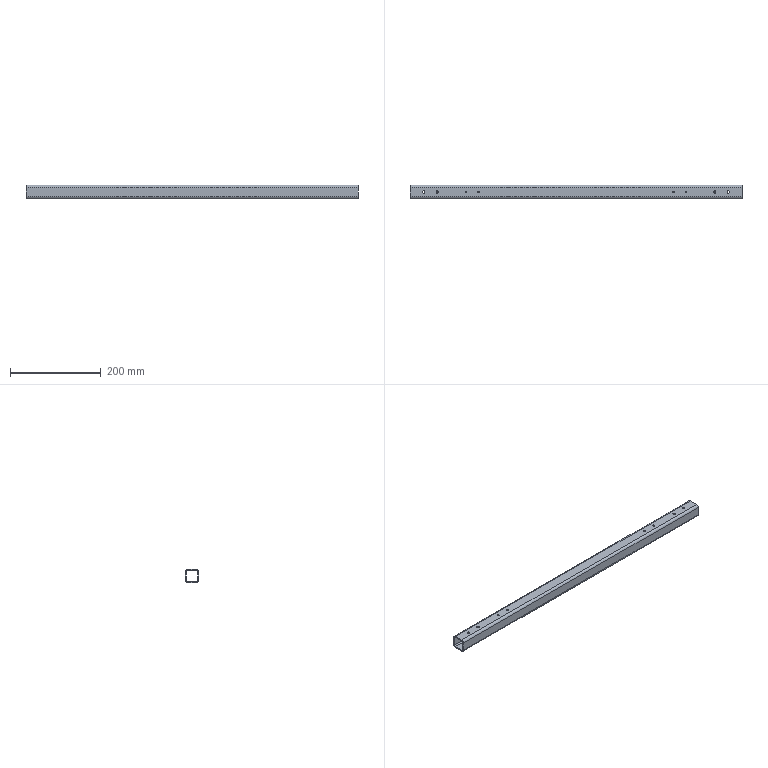Part | SolidWorks | features HoleWzd 2, 3DProfileFeature 1, WeldMemberFeat 1, WeldmentFeature 1 | 1 solid | 50 faces | box 730 x 30 x 30 mm | volume 194616 mm3 | cylinder 40 | plane 10 | commonest cylinder face diameters 4.2 x16 5 x16 5.2 x4 10.4 x4